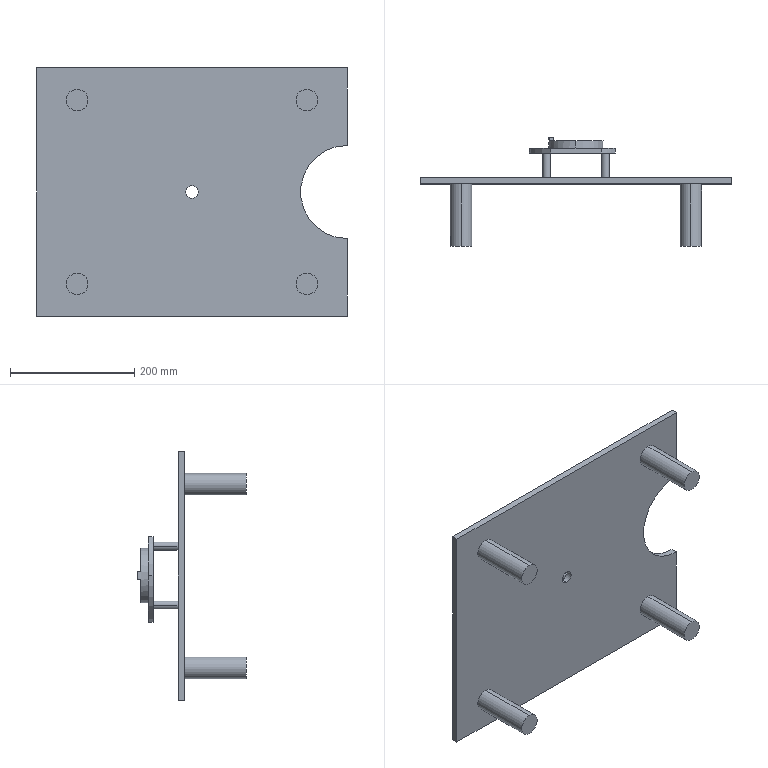Part | SolidWorks | features ICE 2, BaseBody 1 | 1 solid | 49 faces | box 500 x 175 x 400 mm | volume 2505450 mm3 | cylinder 29 | plane 20 | commonest cylinder face diameters 13 x8 35 x8 150 x4 20 x2 29 x2 30 x2
STEP:
#1=CARTESIAN_POINT('',(-15.,50.,0.6238));
#2=VERTEX_POINT('',#1);
#3=CARTESIAN_POINT('',(15.,50.,0.6238));
#4=VERTEX_POINT('',#3);
#5=CARTESIAN_POINT('',(0.,50.,0.6238));
#6=DIRECTION('',(0.,-1.,0.));
#7=DIRECTION('',(1.,0.,0.));
#8=AXIS2_PLACEMENT_3D('',#5,#6,#7);
#9=CIRCLE('',#8,15.);
#10=EDGE_CURVE('',#2,#4,#9,.T.);
#11=ORIENTED_EDGE('',*,*,#10,.T.);
#12=CARTESIAN_POINT('',(15.,58.,0.6238));
#13=VERTEX_POINT('',#12);
#14=CARTESIAN_POINT('',(15.,10.,0.6238));
#15=DIRECTION('',(0.,1.,0.));
#16=VECTOR('',#15,1000.);
#17=LINE('',#14,#16);
#18=EDGE_CURVE('',#4,#13,#17,.T.);
#19=ORIENTED_EDGE('',*,*,#18,.T.);
#20=CARTESIAN_POINT('',(-15.,58.,0.6238));
#21=VERTEX_POINT('',#20);
#22=CARTESIAN_POINT('',(0.,58.,0.6238));
#23=DIRECTION('',(0.,1.,0.));
#24=DIRECTION('',(-1.,0.,0.));
#25=AXIS2_PLACEMENT_3D('',#22,#23,#24);
#26=CIRCLE('',#25,15.);
#27=EDGE_CURVE('',#13,#21,#26,.T.);
#28=ORIENTED_EDGE('',*,*,#27,.T.);
#29=CARTESIAN_POINT('',(-15.,10.,0.6238));
#30=DIRECTION('',(0.,1.,0.));
#31=VECTOR('',#30,1000.);
#32=LINE('',#29,#31);
#33=EDGE_CURVE('',#2,#21,#32,.T.);
#34=ORIENTED_EDGE('',*,*,#33,.F.);
#35=EDGE_LOOP('',(#11,#19,#28,#34));
#36=FACE_OUTER_BOUND('',#35,.T.);
#37=CARTESIAN_POINT('',(0.,10.,0.6238));
#38=DIRECTION('',(0.,1.,0.));
#39=DIRECTION('',(-1.,0.,0.));
#40=AXIS2_PLACEMENT_3D('',#37,#38,#39);
#41=CYLINDRICAL_SURFACE('',#40,15.);
#42=ADVANCED_FACE('',(#36),#41,.F.);
#43=CARTESIAN_POINT('',(-40.876,10.,48.));
#44=VERTEX_POINT('',#43);
#45=CARTESIAN_POINT('',(-53.876,10.,48.));
#46=VERTEX_POINT('',#45);
#47=CARTESIAN_POINT('',(-47.376,10.,48.));
#48=DIRECTION('',(0.,-1.,0.));
#49=DIRECTION('',(1.,0.,0.));
#50=AXIS2_PLACEMENT_3D('',#47,#48,#49);
#51=CIRCLE('',#50,6.5);
#52=EDGE_CURVE('',#44,#46,#51,.T.);
#53=ORIENTED_EDGE('',*,*,#52,.F.);
#54=CARTESIAN_POINT('',(-40.876,50.,48.));
#55=VERTEX_POINT('',#54);
#56=CARTESIAN_POINT('',(-40.876,10.,48.));
#57=DIRECTION('',(0.,1.,0.));
#58=VECTOR('',#57,1000.);
#59=LINE('',#56,#58);
#60=EDGE_CURVE('',#44,#55,#59,.T.);
#61=ORIENTED_EDGE('',*,*,#60,.T.);
#62=CARTESIAN_POINT('',(-53.876,50.,48.));
#63=VERTEX_POINT('',#62);
#64=CARTESIAN_POINT('',(-47.376,50.,48.));
#65=DIRECTION('',(0.,-1.,0.));
#66=DIRECTION('',(1.,0.,0.));
#67=AXIS2_PLACEMENT_3D('',#64,#65,#66);
#68=CIRCLE('',#67,6.5);
#69=EDGE_CURVE('',#55,#63,#68,.T.);
#70=ORIENTED_EDGE('',*,*,#69,.T.);
#71=CARTESIAN_POINT('',(-53.876,10.,48.));
#72=DIRECTION('',(0.,1.,0.));
#73=VECTOR('',#72,1000.);
#74=LINE('',#71,#73);
#75=EDGE_CURVE('',#46,#63,#74,.T.);
#76=ORIENTED_EDGE('',*,*,#75,.F.);
#77=EDGE_LOOP('',(#53,#61,#70,#76));
#78=FACE_OUTER_BOUND('',#77,.T.);
#79=CARTESIAN_POINT('',(-47.376,10.,48.));
#80=DIRECTION('',(0.,1.,0.));
#81=DIRECTION('',(-1.,0.,0.));
#82=AXIS2_PLACEMENT_3D('',#79,#80,#81);
#83=CYLINDRICAL_SURFACE('',#82,6.5);
#84=ADVANCED_FACE('',(#78),#83,.T.);
#85=CARTESIAN_POINT('',(-75.,50.,0.6238));
#86=VERTEX_POINT('',#85);
#87=CARTESIAN_POINT('',(63.5,50.,-39.285));
#88=VERTEX_POINT('',#87);
#89=CARTESIAN_POINT('',(0.,50.,0.6238));
#90=DIRECTION('',(0.,-1.,0.));
#91=DIRECTION('',(1.,0.,0.));
#92=AXIS2_PLACEMENT_3D('',#89,#90,#91);
#93=CIRCLE('',#92,75.);
#94=EDGE_CURVE('',#86,#88,#93,.T.);
#95=ORIENTED_EDGE('',*,*,#94,.F.);
#96=CARTESIAN_POINT('',(-75.,58.,0.6238));
#97=VERTEX_POINT('',#96);
#98=CARTESIAN_POINT('',(-75.,50.,0.6238));
#99=DIRECTION('',(0.,1.,0.));
#100=VECTOR('',#99,1000.);
#101=LINE('',#98,#100);
#102=EDGE_CURVE('',#86,#97,#101,.T.);
#103=ORIENTED_EDGE('',*,*,#102,.T.);
#104=CARTESIAN_POINT('',(63.5,58.,-39.285));
#105=VERTEX_POINT('',#104);
#106=CARTESIAN_POINT('',(0.,58.,0.6238));
#107=DIRECTION('',(0.,-1.,0.));
#108=DIRECTION('',(1.,0.,0.));
#109=AXIS2_PLACEMENT_3D('',#106,#107,#108);
#110=CIRCLE('',#109,75.);
#111=EDGE_CURVE('',#97,#105,#110,.T.);
#112=ORIENTED_EDGE('',*,*,#111,.T.);
#113=CARTESIAN_POINT('',(63.5,50.,-39.285));
#114=DIRECTION('',(0.,-1.,0.));
#115=VECTOR('',#114,1000.);
#116=LINE('',#113,#115);
#117=EDGE_CURVE('',#105,#88,#116,.T.);
#118=ORIENTED_EDGE('',*,*,#117,.T.);
#119=EDGE_LOOP('',(#95,#103,#112,#118));
#120=FACE_OUTER_BOUND('',#119,.T.);
#121=CARTESIAN_POINT('',(0.,50.,0.6238));
#122=DIRECTION('',(0.,1.,0.));
#123=DIRECTION('',(-1.,0.,0.));
#124=AXIS2_PLACEMENT_3D('',#121,#122,#123);
#125=CYLINDRICAL_SURFACE('',#124,75.);
#126=ADVANCED_FACE('',(#120),#125,.T.);
#127=CARTESIAN_POINT('',(-40.876,10.,-46.752));
#128=VERTEX_POINT('',#127);
#129=CARTESIAN_POINT('',(-53.876,10.,-46.752));
#130=VERTEX_POINT('',#129);
#131=CARTESIAN_POINT('',(-47.376,10.,-46.752));
#132=DIRECTION('',(0.,-1.,0.));
#133=DIRECTION('',(0.,0.,1.));
#134=AXIS2_PLACEMENT_3D('',#131,#132,#133);
#135=CIRCLE('',#134,6.5);
#136=EDGE_CURVE('',#128,#130,#135,.T.);
#137=ORIENTED_EDGE('',*,*,#136,.F.);
#138=CARTESIAN_POINT('',(-40.876,50.,-46.752));
#139=VERTEX_POINT('',#138);
#140=CARTESIAN_POINT('',(-40.876,10.,-46.752));
#141=DIRECTION('',(0.,1.,0.));
#142=VECTOR('',#141,1000.);
#143=LINE('',#140,#142);
#144=EDGE_CURVE('',#128,#139,#143,.T.);
#145=ORIENTED_EDGE('',*,*,#144,.T.);
#146=CARTESIAN_POINT('',(-53.876,50.,-46.752));
#147=VERTEX_POINT('',#146);
#148=CARTESIAN_POINT('',(-47.376,50.,-46.752));
#149=DIRECTION('',(0.,-1.,0.));
#150=DIRECTION('',(0.,0.,1.));
#151=AXIS2_PLACEMENT_3D('',#148,#149,#150);
#152=CIRCLE('',#151,6.5);
#153=EDGE_CURVE('',#139,#147,#152,.T.);
#154=ORIENTED_EDGE('',*,*,#153,.T.);
#155=CARTESIAN_POINT('',(-53.876,10.,-46.752));
#156=DIRECTION('',(0.,1.,0.));
#157=VECTOR('',#156,1000.);
#158=LINE('',#155,#157);
#159=EDGE_CURVE('',#130,#147,#158,.T.);
#160=ORIENTED_EDGE('',*,*,#159,.F.);
#161=EDGE_LOOP('',(#137,#145,#154,#160));
#162=FACE_OUTER_BOUND('',#161,.T.);
#163=CARTESIAN_POINT('',(-47.376,10.,-46.752));
#164=DIRECTION('',(0.,1.,0.));
#165=DIRECTION('',(-1.,0.,0.));
#166=AXIS2_PLACEMENT_3D('',#163,#164,#165);
#167=CYLINDRICAL_SURFACE('',#166,6.5);
#168=ADVANCED_FACE('',(#162),#167,.T.);
#169=CARTESIAN_POINT('',(53.876,10.,-46.752));
#170=VERTEX_POINT('',#169);
#171=CARTESIAN_POINT('',(40.876,10.,-46.752));
#172=VERTEX_POINT('',#171);
#173=CARTESIAN_POINT('',(47.376,10.,-46.752));
#174=DIRECTION('',(0.,-1.,0.));
#175=DIRECTION('',(-1.,0.,0.));
#176=AXIS2_PLACEMENT_3D('',#173,#174,#175);
#177=CIRCLE('',#176,6.5);
#178=EDGE_CURVE('',#170,#172,#177,.T.);
#179=ORIENTED_EDGE('',*,*,#178,.F.);
#180=CARTESIAN_POINT('',(53.876,50.,-46.752));
#181=VERTEX_POINT('',#180);
#182=CARTESIAN_POINT('',(53.876,10.,-46.752));
#183=DIRECTION('',(0.,1.,0.));
#184=VECTOR('',#183,1000.);
#185=LINE('',#182,#184);
#186=EDGE_CURVE('',#170,#181,#185,.T.);
#187=ORIENTED_EDGE('',*,*,#186,.T.);
#188=CARTESIAN_POINT('',(40.876,50.,-46.752));
#189=VERTEX_POINT('',#188);
#190=CARTESIAN_POINT('',(47.376,50.,-46.752));
#191=DIRECTION('',(0.,-1.,0.));
#192=DIRECTION('',(-1.,0.,0.));
#193=AXIS2_PLACEMENT_3D('',#190,#191,#192);
#194=CIRCLE('',#193,6.5);
#195=EDGE_CURVE('',#181,#189,#194,.T.);
#196=ORIENTED_EDGE('',*,*,#195,.T.);
#197=CARTESIAN_POINT('',(40.876,10.,-46.752));
#198=DIRECTION('',(0.,1.,0.));
#199=VECTOR('',#198,1000.);
#200=LINE('',#197,#199);
#201=EDGE_CURVE('',#172,#189,#200,.T.);
#202=ORIENTED_EDGE('',*,*,#201,.F.);
#203=EDGE_LOOP('',(#179,#187,#196,#202));
#204=FACE_OUTER_BOUND('',#203,.T.);
#205=CARTESIAN_POINT('',(47.376,10.,-46.752));
#206=DIRECTION('',(0.,1.,0.));
#207=DIRECTION('',(-1.,0.,0.));
#208=AXIS2_PLACEMENT_3D('',#205,#206,#207);
#209=CYLINDRICAL_SURFACE('',#208,6.5);
#210=ADVANCED_FACE('',(#204),#209,.T.);
#211=CARTESIAN_POINT('',(53.876,10.,48.));
#212=VERTEX_POINT('',#211);
#213=CARTESIAN_POINT('',(40.876,10.,48.));
#214=VERTEX_POINT('',#213);
#215=CARTESIAN_POINT('',(47.376,10.,48.));
#216=DIRECTION('',(0.,-1.,0.));
#217=DIRECTION('',(0.,0.,-1.));
#218=AXIS2_PLACEMENT_3D('',#215,#216,#217);
#219=CIRCLE('',#218,6.5);
#220=EDGE_CURVE('',#212,#214,#219,.T.);
#221=ORIENTED_EDGE('',*,*,#220,.F.);
#222=CARTESIAN_POINT('',(53.876,50.,48.));
#223=VERTEX_POINT('',#222);
#224=CARTESIAN_POINT('',(53.876,10.,48.));
#225=DIRECTION('',(0.,1.,0.));
#226=VECTOR('',#225,1000.);
#227=LINE('',#224,#226);
#228=EDGE_CURVE('',#212,#223,#227,.T.);
#229=ORIENTED_EDGE('',*,*,#228,.T.);
#230=CARTESIAN_POINT('',(40.876,50.,48.));
#231=VERTEX_POINT('',#230);
#232=CARTESIAN_POINT('',(47.376,50.,48.));
#233=DIRECTION('',(0.,-1.,0.));
#234=DIRECTION('',(0.,0.,-1.));
#235=AXIS2_PLACEMENT_3D('',#232,#233,#234);
#236=CIRCLE('',#235,6.5);
#237=EDGE_CURVE('',#223,#231,#236,.T.);
#238=ORIENTED_EDGE('',*,*,#237,.T.);
#239=CARTESIAN_POINT('',(40.876,10.,48.));
#240=DIRECTION('',(0.,1.,0.));
#241=VECTOR('',#240,1000.);
#242=LINE('',#239,#241);
#243=EDGE_CURVE('',#214,#231,#242,.T.);
#244=ORIENTED_EDGE('',*,*,#243,.F.);
#245=EDGE_LOOP('',(#221,#229,#238,#244));
#246=FACE_OUTER_BOUND('',#245,.T.);
#247=CARTESIAN_POINT('',(47.376,10.,48.));
#248=DIRECTION('',(0.,1.,0.));
#249=DIRECTION('',(-1.,0.,0.));
#250=AXIS2_PLACEMENT_3D('',#247,#248,#249);
#251=CYLINDRICAL_SURFACE('',#250,6.5);
#252=ADVANCED_FACE('',(#246),#251,.T.);
#253=CARTESIAN_POINT('',(0.,0.,10.));
#254=VERTEX_POINT('',#253);
#255=CARTESIAN_POINT('',(0.,0.,-10.));
#256=VERTEX_POINT('',#255);
#257=CARTESIAN_POINT('',(0.,0.,0.));
#258=DIRECTION('',(0.,-1.,0.));
#259=DIRECTION('',(0.,0.,-1.));
#260=AXIS2_PLACEMENT_3D('',#257,#258,#259);
#261=CIRCLE('',#260,10.);
#262=EDGE_CURVE('',#254,#256,#261,.T.);
#263=ORIENTED_EDGE('',*,*,#262,.T.);
#264=CARTESIAN_POINT('',(0.,10.,-10.));
#265=VERTEX_POINT('',#264);
#266=CARTESIAN_POINT('',(0.,-100.,-10.));
#267=DIRECTION('',(0.,1.,0.));
#268=VECTOR('',#267,1000.);
#269=LINE('',#266,#268);
#270=EDGE_CURVE('',#256,#265,#269,.T.);
#271=ORIENTED_EDGE('',*,*,#270,.T.);
#272=CARTESIAN_POINT('',(0.,10.,10.));
#273=VERTEX_POINT('',#272);
#274=CARTESIAN_POINT('',(0.,10.,0.));
#275=DIRECTION('',(0.,1.,0.));
#276=DIRECTION('',(0.,0.,1.));
#277=AXIS2_PLACEMENT_3D('',#274,#275,#276);
#278=CIRCLE('',#277,10.);
#279=EDGE_CURVE('',#265,#273,#278,.T.);
#280=ORIENTED_EDGE('',*,*,#279,.T.);
#281=CARTESIAN_POINT('',(0.,-100.,10.));
#282=DIRECTION('',(0.,1.,0.));
#283=VECTOR('',#282,1000.);
#284=LINE('',#281,#283);
#285=EDGE_CURVE('',#254,#273,#284,.T.);
#286=ORIENTED_EDGE('',*,*,#285,.F.);
#287=EDGE_LOOP('',(#263,#271,#280,#286));
#288=FACE_OUTER_BOUND('',#287,.T.);
#289=CARTESIAN_POINT('',(0.,-100.,0.));
#290=DIRECTION('',(0.,1.,0.));
#291=DIRECTION('',(0.,0.,1.));
#292=AXIS2_PLACEMENT_3D('',#289,#290,#291);
#293=CYLINDRICAL_SURFACE('',#292,10.);
#294=ADVANCED_FACE('',(#288),#293,.F.);
#295=CARTESIAN_POINT('',(-185.,-100.,165.5));
#296=VERTEX_POINT('',#295);
#297=CARTESIAN_POINT('',(-185.,-100.,130.5));
#298=VERTEX_POINT('',#297);
#299=CARTESIAN_POINT('',(-185.,-100.,148.));
#300=DIRECTION('',(0.,1.,0.));
#301=DIRECTION('',(0.,0.,1.));
#302=AXIS2_PLACEMENT_3D('',#299,#300,#301);
#303=CIRCLE('',#302,17.5);
#304=EDGE_CURVE('',#296,#298,#303,.T.);
#305=ORIENTED_EDGE('',*,*,#304,.T.);
#306=CARTESIAN_POINT('',(-185.,0.,130.5));
#307=VERTEX_POINT('',#306);
#308=CARTESIAN_POINT('',(-185.,-100.,130.5));
#309=DIRECTION('',(0.,1.,0.));
#310=VECTOR('',#309,1000.);
#311=LINE('',#308,#310);
#312=EDGE_CURVE('',#298,#307,#311,.T.);
#313=ORIENTED_EDGE('',*,*,#312,.T.);
#314=CARTESIAN_POINT('',(-185.,0.,165.5));
#315=VERTEX_POINT('',#314);
#316=CARTESIAN_POINT('',(-185.,0.,148.));
#317=DIRECTION('',(0.,-1.,0.));
#318=DIRECTION('',(0.,0.,-1.));
#319=AXIS2_PLACEMENT_3D('',#316,#317,#318);
#320=CIRCLE('',#319,17.5);
#321=EDGE_CURVE('',#307,#315,#320,.T.);
#322=ORIENTED_EDGE('',*,*,#321,.T.);
#323=CARTESIAN_POINT('',(-185.,-100.,165.5));
#324=DIRECTION('',(0.,1.,0.));
#325=VECTOR('',#324,1000.);
#326=LINE('',#323,#325);
#327=EDGE_CURVE('',#296,#315,#326,.T.);
#328=ORIENTED_EDGE('',*,*,#327,.F.);
#329=EDGE_LOOP('',(#305,#313,#322,#328));
#330=FACE_OUTER_BOUND('',#329,.T.);
#331=CARTESIAN_POINT('',(-185.,-100.,148.));
#332=DIRECTION('',(0.,1.,0.));
#333=DIRECTION('',(0.,0.,1.));
#334=AXIS2_PLACEMENT_3D('',#331,#332,#333);
#335=CYLINDRICAL_SURFACE('',#334,17.5);
#336=ADVANCED_FACE('',(#330),#335,.T.);
#337=CARTESIAN_POINT('',(185.,-100.,130.5));
#338=VERTEX_POINT('',#337);
#339=CARTESIAN_POINT('',(185.,-100.,165.5));
#340=VERTEX_POINT('',#339);
#341=CARTESIAN_POINT('',(185.,-100.,148.));
#342=DIRECTION('',(0.,-1.,0.));
#343=DIRECTION('',(0.,0.,1.));
#344=AXIS2_PLACEMENT_3D('',#341,#342,#343);
#345=CIRCLE('',#344,17.5);
#346=EDGE_CURVE('',#338,#340,#345,.T.);
#347=ORIENTED_EDGE('',*,*,#346,.F.);
#348=CARTESIAN_POINT('',(185.,0.,130.5));
#349=VERTEX_POINT('',#348);
#350=CARTESIAN_POINT('',(185.,-100.,130.5));
#351=DIRECTION('',(0.,1.,0.));
#352=VECTOR('',#351,1000.);
#353=LINE('',#350,#352);
#354=EDGE_CURVE('',#338,#349,#353,.T.);
#355=ORIENTED_EDGE('',*,*,#354,.T.);
#356=CARTESIAN_POINT('',(185.,0.,165.5));
#357=VERTEX_POINT('',#356);
#358=CARTESIAN_POINT('',(185.,0.,148.));
#359=DIRECTION('',(0.,-1.,0.));
#360=DIRECTION('',(0.,0.,1.));
#361=AXIS2_PLACEMENT_3D('',#358,#359,#360);
#362=CIRCLE('',#361,17.5);
#363=EDGE_CURVE('',#349,#357,#362,.T.);
#364=ORIENTED_EDGE('',*,*,#363,.T.);
#365=CARTESIAN_POINT('',(185.,-100.,165.5));
#366=DIRECTION('',(0.,1.,0.));
#367=VECTOR('',#366,1000.);
#368=LINE('',#365,#367);
#369=EDGE_CURVE('',#340,#357,#368,.T.);
#370=ORIENTED_EDGE('',*,*,#369,.F.);
#371=EDGE_LOOP('',(#347,#355,#364,#370));
#372=FACE_OUTER_BOUND('',#371,.T.);
#373=CARTESIAN_POINT('',(185.,-100.,148.));
#374=DIRECTION('',(0.,1.,0.));
#375=DIRECTION('',(0.,0.,1.));
#376=AXIS2_PLACEMENT_3D('',#373,#374,#375);
#377=CYLINDRICAL_SURFACE('',#376,17.5);
#378=ADVANCED_FACE('',(#372),#377,.T.);
#379=CARTESIAN_POINT('',(185.,-100.,-130.5));
#380=VERTEX_POINT('',#379);
#381=CARTESIAN_POINT('',(185.,-100.,-165.5));
#382=VERTEX_POINT('',#381);
#383=CARTESIAN_POINT('',(185.,-100.,-148.));
#384=DIRECTION('',(0.,1.,0.));
#385=DIRECTION('',(0.,0.,-1.));
#386=AXIS2_PLACEMENT_3D('',#383,#384,#385);
#387=CIRCLE('',#386,17.5);
#388=EDGE_CURVE('',#380,#382,#387,.T.);
#389=ORIENTED_EDGE('',*,*,#388,.T.);
#390=CARTESIAN_POINT('',(185.,0.,-165.5));
#391=VERTEX_POINT('',#390);
#392=CARTESIAN_POINT('',(185.,-100.,-165.5));
#393=DIRECTION('',(0.,1.,0.));
#394=VECTOR('',#393,1000.);
#395=LINE('',#392,#394);
#396=EDGE_CURVE('',#382,#391,#395,.T.);
#397=ORIENTED_EDGE('',*,*,#396,.T.);
#398=CARTESIAN_POINT('',(185.,0.,-130.5));
#399=VERTEX_POINT('',#398);
#400=CARTESIAN_POINT('',(185.,0.,-148.));
#401=DIRECTION('',(0.,-1.,0.));
#402=DIRECTION('',(0.,0.,-1.));
#403=AXIS2_PLACEMENT_3D('',#400,#401,#402);
#404=CIRCLE('',#403,17.5);
#405=EDGE_CURVE('',#391,#399,#404,.T.);
#406=ORIENTED_EDGE('',*,*,#405,.T.);
#407=CARTESIAN_POINT('',(185.,-100.,-130.5));
#408=DIRECTION('',(0.,1.,0.));
#409=VECTOR('',#408,1000.);
#410=LINE('',#407,#409);
#411=EDGE_CURVE('',#380,#399,#410,.T.);
#412=ORIENTED_EDGE('',*,*,#411,.F.);
#413=EDGE_LOOP('',(#389,#397,#406,#412));
#414=FACE_OUTER_BOUND('',#413,.T.);
#415=CARTESIAN_POINT('',(185.,-100.,-148.));
#416=DIRECTION('',(0.,1.,0.));
#417=DIRECTION('',(0.,0.,1.));
#418=AXIS2_PLACEMENT_3D('',#415,#416,#417);
#419=CYLINDRICAL_SURFACE('',#418,17.5);
#420=ADVANCED_FACE('',(#414),#419,.T.);
#421=CARTESIAN_POINT('',(-185.,-100.,-165.5));
#422=VERTEX_POINT('',#421);
#423=CARTESIAN_POINT('',(-185.,-100.,-130.5));
#424=VERTEX_POINT('',#423);
#425=CARTESIAN_POINT('',(-185.,-100.,-148.));
#426=DIRECTION('',(0.,-1.,0.));
#427=DIRECTION('',(0.,0.,-1.));
#428=AXIS2_PLACEMENT_3D('',#425,#426,#427);
#429=CIRCLE('',#428,17.5);
#430=EDGE_CURVE('',#422,#424,#429,.T.);
#431=ORIENTED_EDGE('',*,*,#430,.F.);
#432=CARTESIAN_POINT('',(-185.,0.,-165.5));
#433=VERTEX_POINT('',#432);
#434=CARTESIAN_POINT('',(-185.,-100.,-165.5));
#435=DIRECTION('',(0.,1.,0.));
#436=VECTOR('',#435,1000.);
#437=LINE('',#434,#436);
#438=EDGE_CURVE('',#422,#433,#437,.T.);
#439=ORIENTED_EDGE('',*,*,#438,.T.);
#440=CARTESIAN_POINT('',(-185.,0.,-130.5));
#441=VERTEX_POINT('',#440);
#442=CARTESIAN_POINT('',(-185.,0.,-148.));
#443=DIRECTION('',(0.,-1.,0.));
#444=DIRECTION('',(0.,0.,-1.));
#445=AXIS2_PLACEMENT_3D('',#442,#443,#444);
#446=CIRCLE('',#445,17.5);
#447=EDGE_CURVE('',#433,#441,#446,.T.);
#448=ORIENTED_EDGE('',*,*,#447,.T.);
#449=CARTESIAN_POINT('',(-185.,-100.,-130.5));
#450=DIRECTION('',(0.,1.,0.));
#451=VECTOR('',#450,1000.);
#452=LINE('',#449,#451);
#453=EDGE_CURVE('',#424,#441,#452,.T.);
#454=ORIENTED_EDGE('',*,*,#453,.F.);
#455=EDGE_LOOP('',(#431,#439,#448,#454));
#456=FACE_OUTER_BOUND('',#455,.T.);
#457=CARTESIAN_POINT('',(-185.,-100.,-148.));
#458=DIRECTION('',(0.,1.,0.));
#459=DIRECTION('',(0.,0.,1.));
#460=AXIS2_PLACEMENT_3D('',#457,#458,#459);
#461=CYLINDRICAL_SURFACE('',#460,17.5);
#462=ADVANCED_FACE('',(#456),#461,.T.);
#463=CARTESIAN_POINT('',(0.,70.,15.124));
#464=VERTEX_POINT('',#463);
#465=CARTESIAN_POINT('',(0.,70.,-13.876));
#466=VERTEX_POINT('',#465);
#467=CARTESIAN_POINT('',(0.,70.,0.6238));
#468=DIRECTION('',(0.,-1.,0.));
#469=DIRECTION('',(0.,0.,-1.));
#470=AXIS2_PLACEMENT_3D('',#467,#468,#469);
#471=CIRCLE('',#470,14.5);
#472=EDGE_CURVE('',#464,#466,#471,.T.);
#473=ORIENTED_EDGE('',*,*,#472,.F.);
#474=CARTESIAN_POINT('',(0.,58.,15.124));
#475=VERTEX_POINT('',#474);
#476=CARTESIAN_POINT('',(0.,58.,15.124));
#477=DIRECTION('',(0.,-1.,0.));
#478=VECTOR('',#477,1000.);
#479=LINE('',#476,#478);
#480=EDGE_CURVE('',#464,#475,#479,.T.);
#481=ORIENTED_EDGE('',*,*,#480,.T.);
#482=CARTESIAN_POINT('',(0.,58.,-13.876));
#483=VERTEX_POINT('',#482);
#484=CARTESIAN_POINT('',(0.,58.,0.6238));
#485=DIRECTION('',(0.,-1.,0.));
#486=DIRECTION('',(0.,0.,-1.));
#487=AXIS2_PLACEMENT_3D('',#484,#485,#486);
#488=CIRCLE('',#487,14.5);
#489=EDGE_CURVE('',#475,#483,#488,.T.);
#490=ORIENTED_EDGE('',*,*,#489,.T.);
#491=CARTESIAN_POINT('',(0.,58.,-13.876));
#492=DIRECTION('',(0.,-1.,0.));
#493=VECTOR('',#492,1000.);
#494=LINE('',#491,#493);
#495=EDGE_CURVE('',#466,#483,#494,.T.);
#496=ORIENTED_EDGE('',*,*,#495,.F.);
#497=EDGE_LOOP('',(#473,#481,#490,#496));
#498=FACE_OUTER_BOUND('',#497,.T.);
#499=CARTESIAN_POINT('',(0.,58.,0.6238));
#500=DIRECTION('',(0.,-1.,0.));
#501=DIRECTION('',(0.,0.,-1.));
#502=AXIS2_PLACEMENT_3D('',#499,#500,#501);
#503=CYLINDRICAL_SURFACE('',#502,14.5);
#504=ADVANCED_FACE('',(#498),#503,.F.);
#505=CARTESIAN_POINT('',(0.,70.,-43.376));
#506=VERTEX_POINT('',#505);
#507=CARTESIAN_POINT('',(0.,70.,44.624));
#508=VERTEX_POINT('',#507);
#509=CARTESIAN_POINT('',(0.,70.,0.6238));
#510=DIRECTION('',(0.,-1.,0.));
#511=DIRECTION('',(0.,0.,-1.));
#512=AXIS2_PLACEMENT_3D('',#509,#510,#511);
#513=CIRCLE('',#512,44.);
#514=EDGE_CURVE('',#506,#508,#513,.T.);
#515=ORIENTED_EDGE('',*,*,#514,.T.);
#516=CARTESIAN_POINT('',(0.,58.,44.624));
#517=VERTEX_POINT('',#516);
#518=CARTESIAN_POINT('',(0.,58.,44.624));
#519=DIRECTION('',(0.,-1.,0.));
#520=VECTOR('',#519,1000.);
#521=LINE('',#518,#520);
#522=EDGE_CURVE('',#508,#517,#521,.T.);
#523=ORIENTED_EDGE('',*,*,#522,.T.);
#524=CARTESIAN_POINT('',(0.,58.,-43.376));
#525=VERTEX_POINT('',#524);
#526=CARTESIAN_POINT('',(0.,58.,0.6238));
#527=DIRECTION('',(0.,-1.,0.));
#528=DIRECTION('',(0.,0.,-1.));
#529=AXIS2_PLACEMENT_3D('',#526,#527,#528);
#530=CIRCLE('',#529,44.);
#531=EDGE_CURVE('',#525,#517,#530,.T.);
#532=ORIENTED_EDGE('',*,*,#531,.F.);
#533=CARTESIAN_POINT('',(0.,58.,-43.376));
#534=DIRECTION('',(0.,-1.,0.));
#535=VECTOR('',#534,1000.);
#536=LINE('',#533,#535);
#537=EDGE_CURVE('',#506,#525,#536,.T.);
#538=ORIENTED_EDGE('',*,*,#537,.F.);
#539=EDGE_LOOP('',(#515,#523,#532,#538));
#540=FACE_OUTER_BOUND('',#539,.T.);
#541=CARTESIAN_POINT('',(0.,58.,0.6238));
#542=DIRECTION('',(0.,-1.,0.));
#543=DIRECTION('',(0.,0.,-1.));
#544=AXIS2_PLACEMENT_3D('',#541,#542,#543);
#545=CYLINDRICAL_SURFACE('',#544,44.);
#546=ADVANCED_FACE('',(#540),#545,.T.);
#547=CARTESIAN_POINT('',(250.,0.,200.));
#548=VERTEX_POINT('',#547);
#549=CARTESIAN_POINT('',(250.,0.,75.));
#550=VERTEX_POINT('',#549);
#551=CARTESIAN_POINT('',(250.,0.,-200.));
#552=DIRECTION('',(0.,0.,-1.));
#553=VECTOR('',#552,1000.);
#554=LINE('',#551,#553);
#555=EDGE_CURVE('',#548,#550,#554,.T.);
#556=ORIENTED_EDGE('',*,*,#555,.T.);
#557=CARTESIAN_POINT('',(250.,10.,75.));
#558=VERTEX_POINT('',#557);
#559=CARTESIAN_POINT('',(250.,-100.,75.));
#560=DIRECTION('',(0.,1.,0.));
#561=VECTOR('',#560,1000.);
#562=LINE('',#559,#561);
#563=EDGE_CURVE('',#550,#558,#562,.T.);
#564=ORIENTED_EDGE('',*,*,#563,.T.);
#565=CARTESIAN_POINT('',(250.,10.,200.));
#566=VERTEX_POINT('',#565);
#567=CARTESIAN_POINT('',(250.,10.,200.));
#568=DIRECTION('',(0.,0.,-1.));
#569=VECTOR('',#568,1000.);
#570=LINE('',#567,#569);
#571=EDGE_CURVE('',#566,#558,#570,.T.);
#572=ORIENTED_EDGE('',*,*,#571,.F.);
#573=CARTESIAN_POINT('',(250.,4.,200.));
#574=DIRECTION('',(0.,-1.,0.));
#575=VECTOR('',#574,1000.);
#576=LINE('',#573,#575);
#577=EDGE_CURVE('',#566,#548,#576,.T.);
#578=ORIENTED_EDGE('',*,*,#577,.T.);
#579=EDGE_LOOP('',(#556,#564,#572,#578));
#580=FACE_OUTER_BOUND('',#579,.T.);
#581=CARTESIAN_POINT('',(250.,4.,-200.));
#582=DIRECTION('',(-1.,0.,0.));
#583=DIRECTION('',(0.,0.,1.));
#584=AXIS2_PLACEMENT_3D('',#581,#582,#583);
#585=PLANE('',#584);
#586=ADVANCED_FACE('',(#580),#585,.F.);
#587=CARTESIAN_POINT('',(63.5,50.,40.533));
#588=VERTEX_POINT('',#587);
#589=CARTESIAN_POINT('',(40.885,50.,63.5));
#590=VERTEX_POINT('',#589);
#591=CARTESIAN_POINT('',(0.,50.,0.6238));
#592=DIRECTION('',(0.,-1.,0.));
#593=DIRECTION('',(1.,0.,0.));
#594=AXIS2_PLACEMENT_3D('',#591,#592,#593);
#595=CIRCLE('',#594,75.);
#596=EDGE_CURVE('',#588,#590,#595,.T.);
#597=ORIENTED_EDGE('',*,*,#596,.F.);
#598=CARTESIAN_POINT('',(63.5,58.,40.533));
#599=VERTEX_POINT('',#598);
#600=CARTESIAN_POINT('',(63.5,50.,40.533));
#601=DIRECTION('',(0.,1.,0.));
#602=VECTOR('',#601,1000.);
#603=LINE('',#600,#602);
#604=EDGE_CURVE('',#588,#599,#603,.T.);
#605=ORIENTED_EDGE('',*,*,#604,.T.);
#606=CARTESIAN_POINT('',(40.885,58.,63.5));
#607=VERTEX_POINT('',#606);
#608=CARTESIAN_POINT('',(0.,58.,0.6238));
#609=DIRECTION('',(0.,-1.,0.));
#610=DIRECTION('',(1.,0.,0.));
#611=AXIS2_PLACEMENT_3D('',#608,#609,#610);
#612=CIRCLE('',#611,75.);
#613=EDGE_CURVE('',#599,#607,#612,.T.);
#614=ORIENTED_EDGE('',*,*,#613,.T.);
#615=CARTESIAN_POINT('',(40.885,50.,63.5));
#616=DIRECTION('',(0.,-1.,0.));
#617=VECTOR('',#616,1000.);
#618=LINE('',#615,#617);
#619=EDGE_CURVE('',#607,#590,#618,.T.);
#620=ORIENTED_EDGE('',*,*,#619,.T.);
#621=EDGE_LOOP('',(#597,#605,#614,#620));
#622=FACE_OUTER_BOUND('',#621,.T.);
#623=CARTESIAN_POINT('',(0.,50.,0.6238));
#624=DIRECTION('',(0.,1.,0.));
#625=DIRECTION('',(-1.,0.,0.));
#626=AXIS2_PLACEMENT_3D('',#623,#624,#625);
#627=CYLINDRICAL_SURFACE('',#626,75.);
#628=ADVANCED_FACE('',(#622),#627,.T.);
#629=CARTESIAN_POINT('',(0.,58.,0.6238));
#630=DIRECTION('',(0.,-1.,0.));
#631=DIRECTION('',(0.,0.,-1.));
#632=AXIS2_PLACEMENT_3D('',#629,#630,#631);
#633=CIRCLE('',#632,14.5);
#634=EDGE_CURVE('',#483,#475,#633,.T.);
#635=ORIENTED_EDGE('',*,*,#634,.F.);
#636=ORIENTED_EDGE('',*,*,#489,.F.);
#637=EDGE_LOOP('',(#635,#636));
#638=FACE_BOUND('',#637,.T.);
#639=CARTESIAN_POINT('',(0.,58.,0.6238));
#640=DIRECTION('',(0.,1.,0.));
#641=DIRECTION('',(-1.,0.,0.));
#642=AXIS2_PLACEMENT_3D('',#639,#640,#641);
#643=CIRCLE('',#642,15.);
#644=EDGE_CURVE('',#21,#13,#643,.T.);
#645=ORIENTED_EDGE('',*,*,#644,.F.);
#646=ORIENTED_EDGE('',*,*,#27,.F.);
#647=EDGE_LOOP('',(#645,#646));
#648=FACE_OUTER_BOUND('',#647,.T.);
#649=CARTESIAN_POINT('',(14.5,58.,0.6238));
#650=DIRECTION('',(0.,-1.,0.));
#651=DIRECTION('',(0.,0.,-1.));
#652=AXIS2_PLACEMENT_3D('',#649,#650,#651);
#653=PLANE('',#652);
#654=ADVANCED_FACE('',(#638,#648),#653,.T.);
#655=ORIENTED_EDGE('',*,*,#522,.F.);
#656=CARTESIAN_POINT('',(-43.458,70.,7.507));
#657=VERTEX_POINT('',#656);
#658=CARTESIAN_POINT('',(0.,70.,0.6238));
#659=DIRECTION('',(0.,-1.,0.));
#660=DIRECTION('',(0.,0.,-1.));
#661=AXIS2_PLACEMENT_3D('',#658,#659,#660);
#662=CIRCLE('',#661,44.);
#663=EDGE_CURVE('',#508,#657,#662,.T.);
#664=ORIENTED_EDGE('',*,*,#663,.T.);
#665=CARTESIAN_POINT('',(-43.458,75.,7.507));
#666=VERTEX_POINT('',#665);
#667=CARTESIAN_POINT('',(-43.458,75.,7.507));
#668=DIRECTION('',(0.,-1.,0.));
#669=VECTOR('',#668,1000.);
#670=LINE('',#667,#669);
#671=EDGE_CURVE('',#666,#657,#670,.T.);
#672=ORIENTED_EDGE('',*,*,#671,.F.);
#673=CARTESIAN_POINT('',(-43.458,75.,-6.259));
#674=VERTEX_POINT('',#673);
#675=CARTESIAN_POINT('',(0.,75.,0.6238));
#676=DIRECTION('',(0.,1.,0.));
#677=DIRECTION('',(0.,0.,1.));
#678=AXIS2_PLACEMENT_3D('',#675,#676,#677);
#679=CIRCLE('',#678,44.);
#680=EDGE_CURVE('',#674,#666,#679,.T.);
#681=ORIENTED_EDGE('',*,*,#680,.F.);
#682=CARTESIAN_POINT('',(-43.458,70.,-6.259));
#683=VERTEX_POINT('',#682);
#684=CARTESIAN_POINT('',(-43.458,75.,-6.259));
#685=DIRECTION('',(0.,-1.,0.));
#686=VECTOR('',#685,1000.);
#687=LINE('',#684,#686);
#688=EDGE_CURVE('',#674,#683,#687,.T.);
#689=ORIENTED_EDGE('',*,*,#688,.T.);
#690=CARTESIAN_POINT('',(0.,70.,0.6238));
#691=DIRECTION('',(0.,-1.,0.));
#692=DIRECTION('',(0.,0.,-1.));
#693=AXIS2_PLACEMENT_3D('',#690,#691,#692);
#694=CIRCLE('',#693,44.);
#695=EDGE_CURVE('',#683,#506,#694,.T.);
#696=ORIENTED_EDGE('',*,*,#695,.T.);
#697=ORIENTED_EDGE('',*,*,#537,.T.);
#698=CARTESIAN_POINT('',(0.,58.,0.6238));
#699=DIRECTION('',(0.,-1.,0.));
#700=DIRECTION('',(0.,0.,-1.));
#701=AXIS2_PLACEMENT_3D('',#698,#699,#700);
#702=CIRCLE('',#701,44.);
#703=EDGE_CURVE('',#517,#525,#702,.T.);
#704=ORIENTED_EDGE('',*,*,#703,.F.);
#705=EDGE_LOOP('',(#655,#664,#672,#681,#689,#696,#697,#704));
#706=FACE_OUTER_BOUND('',#705,.T.);
#707=CARTESIAN_POINT('',(0.,58.,0.6238));
#708=DIRECTION('',(0.,-1.,0.));
#709=DIRECTION('',(0.,0.,-1.));
#710=AXIS2_PLACEMENT_3D('',#707,#708,#709);
#711=CYLINDRICAL_SURFACE('',#710,44.);
#712=ADVANCED_FACE('',(#706),#711,.T.);
#713=ORIENTED_EDGE('',*,*,#480,.F.);
#714=CARTESIAN_POINT('',(0.,70.,0.6238));
#715=DIRECTION('',(0.,-1.,0.));
#716=DIRECTION('',(0.,0.,-1.));
#717=AXIS2_PLACEMENT_3D('',#714,#715,#716);
#718=CIRCLE('',#717,14.5);
#719=EDGE_CURVE('',#466,#464,#718,.T.);
#720=ORIENTED_EDGE('',*,*,#719,.F.);
#721=ORIENTED_EDGE('',*,*,#495,.T.);
#722=ORIENTED_EDGE('',*,*,#634,.T.);
#723=EDGE_LOOP('',(#713,#720,#721,#722));
#724=FACE_OUTER_BOUND('',#723,.T.);
#725=CARTESIAN_POINT('',(0.,58.,0.6238));
#726=DIRECTION('',(0.,-1.,0.));
#727=DIRECTION('',(0.,0.,-1.));
#728=AXIS2_PLACEMENT_3D('',#725,#726,#727);
#729=CYLINDRICAL_SURFACE('',#728,14.5);
#730=ADVANCED_FACE('',(#724),#729,.F.);
#731=CARTESIAN_POINT('',(-36.544,70.,-5.164));
#732=VERTEX_POINT('',#731);
#733=CARTESIAN_POINT('',(0.,70.,0.6238));
#734=DIRECTION('',(-0.9877,0.,-0.1564));
#735=VECTOR('',#734,1000.);
#736=LINE('',#733,#735);
#737=EDGE_CURVE('',#732,#683,#736,.T.);
#738=ORIENTED_EDGE('',*,*,#737,.F.);
#739=CARTESIAN_POINT('',(-36.544,70.,6.412));
#740=VERTEX_POINT('',#739);
#741=CARTESIAN_POINT('',(0.,70.,0.6238));
#742=DIRECTION('',(0.,1.,0.));
#743=DIRECTION('',(0.,0.,1.));
#744=AXIS2_PLACEMENT_3D('',#741,#742,#743);
#745=CIRCLE('',#744,37.);
#746=EDGE_CURVE('',#732,#740,#745,.T.);
#747=ORIENTED_EDGE('',*,*,#746,.T.);
#748=CARTESIAN_POINT('',(0.,70.,0.6238));
#749=DIRECTION('',(-0.9877,0.,0.1564));
#750=VECTOR('',#749,1000.);
#751=LINE('',#748,#750);
#752=EDGE_CURVE('',#740,#657,#751,.T.);
#753=ORIENTED_EDGE('',*,*,#752,.T.);
#754=ORIENTED_EDGE('',*,*,#663,.F.);
#755=ORIENTED_EDGE('',*,*,#514,.F.);
#756=ORIENTED_EDGE('',*,*,#695,.F.);
#757=EDGE_LOOP('',(#738,#747,#753,#754,#755,#756));
#758=FACE_OUTER_BOUND('',#757,.T.);
#759=ORIENTED_EDGE('',*,*,#719,.T.);
#760=ORIENTED_EDGE('',*,*,#472,.T.);
#761=EDGE_LOOP('',(#759,#760));
#762=FACE_BOUND('',#761,.T.);
#763=CARTESIAN_POINT('',(14.5,70.,0.6238));
#764=DIRECTION('',(0.,1.,0.));
#765=DIRECTION('',(0.,0.,1.));
#766=AXIS2_PLACEMENT_3D('',#763,#764,#765);
#767=PLANE('',#766);
#768=ADVANCED_FACE('',(#758,#762),#767,.T.);
#769=ORIENTED_EDGE('',*,*,#752,.F.);
#770=CARTESIAN_POINT('',(-36.544,75.,6.412));
#771=VERTEX_POINT('',#770);
#772=CARTESIAN_POINT('',(-36.544,75.,6.412));
#773=DIRECTION('',(0.,-1.,0.));
#774=VECTOR('',#773,1000.);
#775=LINE('',#772,#774);
#776=EDGE_CURVE('',#771,#740,#775,.T.);
#777=ORIENTED_EDGE('',*,*,#776,.F.);
#778=CARTESIAN_POINT('',(0.,75.,0.6238));
#779=DIRECTION('',(-0.9877,0.,0.1564));
#780=VECTOR('',#779,1000.);
#781=LINE('',#778,#780);
#782=EDGE_CURVE('',#771,#666,#781,.T.);
#783=ORIENTED_EDGE('',*,*,#782,.T.);
#784=ORIENTED_EDGE('',*,*,#671,.T.);
#785=EDGE_LOOP('',(#769,#777,#783,#784));
#786=FACE_OUTER_BOUND('',#785,.T.);
#787=CARTESIAN_POINT('',(0.,75.,0.6238));
#788=DIRECTION('',(0.1564,0.,0.9877));
#789=DIRECTION('',(0.9877,0.,-0.1564));
#790=AXIS2_PLACEMENT_3D('',#787,#788,#789);
#791=PLANE('',#790);
#792=ADVANCED_FACE('',(#786),#791,.T.);
#793=ORIENTED_EDGE('',*,*,#746,.F.);
#794=CARTESIAN_POINT('',(-36.544,75.,-5.164));
#795=VERTEX_POINT('',#794);
#796=CARTESIAN_POINT('',(-36.544,75.,-5.164));
#797=DIRECTION('',(0.,-1.,0.));
#798=VECTOR('',#797,1000.);
#799=LINE('',#796,#798);
#800=EDGE_CURVE('',#795,#732,#799,.T.);
#801=ORIENTED_EDGE('',*,*,#800,.F.);
#802=CARTESIAN_POINT('',(0.,75.,0.6238));
#803=DIRECTION('',(0.,1.,0.));
#804=DIRECTION('',(0.,0.,1.));
#805=AXIS2_PLACEMENT_3D('',#802,#803,#804);
#806=CIRCLE('',#805,37.);
#807=EDGE_CURVE('',#795,#771,#806,.T.);
#808=ORIENTED_EDGE('',*,*,#807,.T.);
#809=ORIENTED_EDGE('',*,*,#776,.T.);
#810=EDGE_LOOP('',(#793,#801,#808,#809));
#811=FACE_OUTER_BOUND('',#810,.T.);
#812=CARTESIAN_POINT('',(0.,75.,0.6238));
#813=DIRECTION('',(0.,-1.,0.));
#814=DIRECTION('',(0.,0.,-1.));
#815=AXIS2_PLACEMENT_3D('',#812,#813,#814);
#816=CYLINDRICAL_SURFACE('',#815,37.);
#817=ADVANCED_FACE('',(#811),#816,.F.);
#818=ORIENTED_EDGE('',*,*,#737,.T.);
#819=ORIENTED_EDGE('',*,*,#688,.F.);
#820=CARTESIAN_POINT('',(0.,75.,0.6238));
#821=DIRECTION('',(-0.9877,0.,-0.1564));
#822=VECTOR('',#821,1000.);
#823=LINE('',#820,#822);
#824=EDGE_CURVE('',#795,#674,#823,.T.);
#825=ORIENTED_EDGE('',*,*,#824,.F.);
#826=ORIENTED_EDGE('',*,*,#800,.T.);
#827=EDGE_LOOP('',(#818,#819,#825,#826));
#828=FACE_OUTER_BOUND('',#827,.T.);
#829=CARTESIAN_POINT('',(0.,75.,0.6238));
#830=DIRECTION('',(-0.1564,0.,0.9877));
#831=DIRECTION('',(0.9877,0.,0.1564));
#832=AXIS2_PLACEMENT_3D('',#829,#830,#831);
#833=PLANE('',#832);
#834=ADVANCED_FACE('',(#828),#833,.F.);
#835=ORIENTED_EDGE('',*,*,#680,.T.);
#836=ORIENTED_EDGE('',*,*,#782,.F.);
#837=ORIENTED_EDGE('',*,*,#807,.F.);
#838=ORIENTED_EDGE('',*,*,#824,.T.);
#839=EDGE_LOOP('',(#835,#836,#837,#838));
#840=FACE_OUTER_BOUND('',#839,.T.);
#841=CARTESIAN_POINT('',(0.,75.,0.6238));
#842=DIRECTION('',(0.,1.,0.));
#843=DIRECTION('',(0.,0.,1.));
#844=AXIS2_PLACEMENT_3D('',#841,#842,#843);
#845=PLANE('',#844);
#846=ADVANCED_FACE('',(#840),#845,.T.);
#847=ORIENTED_EDGE('',*,*,#613,.F.);
#848=CARTESIAN_POINT('',(63.5,58.,-50.8));
#849=DIRECTION('',(0.,0.,1.));
#850=VECTOR('',#849,1000.);
#851=LINE('',#848,#850);
#852=EDGE_CURVE('',#105,#599,#851,.T.);
#853=ORIENTED_EDGE('',*,*,#852,.F.);
#854=ORIENTED_EDGE('',*,*,#111,.F.);
#855=CARTESIAN_POINT('',(-40.885,58.,63.5));
#856=VERTEX_POINT('',#855);
#857=CARTESIAN_POINT('',(0.,58.,0.6238));
#858=DIRECTION('',(0.,-1.,0.));
#859=DIRECTION('',(1.,0.,0.));
#860=AXIS2_PLACEMENT_3D('',#857,#858,#859);
#861=CIRCLE('',#860,75.);
#862=EDGE_CURVE('',#856,#97,#861,.T.);
#863=ORIENTED_EDGE('',*,*,#862,.F.);
#864=CARTESIAN_POINT('',(-50.8,58.,63.5));
#865=DIRECTION('',(-1.,0.,0.));
#866=VECTOR('',#865,1000.);
#867=LINE('',#864,#866);
#868=EDGE_CURVE('',#607,#856,#867,.T.);
#869=ORIENTED_EDGE('',*,*,#868,.F.);
#870=EDGE_LOOP('',(#847,#853,#854,#863,#869));
#871=FACE_OUTER_BOUND('',#870,.T.);
#872=ORIENTED_EDGE('',*,*,#531,.T.);
#873=ORIENTED_EDGE('',*,*,#703,.T.);
#874=EDGE_LOOP('',(#872,#873));
#875=FACE_BOUND('',#874,.T.);
#876=CARTESIAN_POINT('',(0.,58.,0.6238));
#877=DIRECTION('',(0.,-1.,0.));
#878=DIRECTION('',(1.,0.,0.));
#879=AXIS2_PLACEMENT_3D('',#876,#877,#878);
#880=PLANE('',#879);
#881=ADVANCED_FACE('',(#871,#875),#880,.F.);
#882=CARTESIAN_POINT('',(250.,0.,-75.));
#883=VERTEX_POINT('',#882);
#884=CARTESIAN_POINT('',(250.,0.,0.));
#885=DIRECTION('',(0.,-1.,0.));
#886=DIRECTION('',(0.,0.,-1.));
#887=AXIS2_PLACEMENT_3D('',#884,#885,#886);
#888=CIRCLE('',#887,75.);
#889=EDGE_CURVE('',#550,#883,#888,.T.);
#890=ORIENTED_EDGE('',*,*,#889,.F.);
#891=ORIENTED_EDGE('',*,*,#555,.F.);
#892=CARTESIAN_POINT('',(-250.,0.,200.));
#893=VERTEX_POINT('',#892);
#894=CARTESIAN_POINT('',(250.,0.,200.));
#895=DIRECTION('',(1.,0.,0.));
#896=VECTOR('',#895,1000.);
#897=LINE('',#894,#896);
#898=EDGE_CURVE('',#893,#548,#897,.T.);
#899=ORIENTED_EDGE('',*,*,#898,.F.);
#900=CARTESIAN_POINT('',(-250.,0.,-200.));
#901=VERTEX_POINT('',#900);
#902=CARTESIAN_POINT('',(-250.,0.,-200.));
#903=DIRECTION('',(0.,0.,1.));
#904=VECTOR('',#903,1000.);
#905=LINE('',#902,#904);
#906=EDGE_CURVE('',#901,#893,#905,.T.);
#907=ORIENTED_EDGE('',*,*,#906,.F.);
#908=CARTESIAN_POINT('',(250.,0.,-200.));
#909=VERTEX_POINT('',#908);
#910=CARTESIAN_POINT('',(250.,0.,-200.));
#911=DIRECTION('',(-1.,0.,0.));
#912=VECTOR('',#911,1000.);
#913=LINE('',#910,#912);
#914=EDGE_CURVE('',#909,#901,#913,.T.);
#915=ORIENTED_EDGE('',*,*,#914,.F.);
#916=CARTESIAN_POINT('',(250.,0.,-200.));
#917=DIRECTION('',(0.,0.,-1.));
#918=VECTOR('',#917,1000.);
#919=LINE('',#916,#918);
#920=EDGE_CURVE('',#883,#909,#919,.T.);
#921=ORIENTED_EDGE('',*,*,#920,.F.);
#922=EDGE_LOOP('',(#890,#891,#899,#907,#915,#921));
#923=FACE_OUTER_BOUND('',#922,.T.);
#924=ORIENTED_EDGE('',*,*,#262,.F.);
#925=CARTESIAN_POINT('',(0.,0.,0.));
#926=DIRECTION('',(0.,-1.,0.));
#927=DIRECTION('',(0.,0.,-1.));
#928=AXIS2_PLACEMENT_3D('',#925,#926,#927);
#929=CIRCLE('',#928,10.);
#930=EDGE_CURVE('',#256,#254,#929,.T.);
#931=ORIENTED_EDGE('',*,*,#930,.F.);
#932=EDGE_LOOP('',(#924,#931));
#933=FACE_BOUND('',#932,.T.);
#934=CARTESIAN_POINT('',(-185.,0.,148.));
#935=DIRECTION('',(0.,-1.,0.));
#936=DIRECTION('',(0.,0.,-1.));
#937=AXIS2_PLACEMENT_3D('',#934,#935,#936);
#938=CIRCLE('',#937,17.5);
#939=EDGE_CURVE('',#315,#307,#938,.T.);
#940=ORIENTED_EDGE('',*,*,#939,.F.);
#941=ORIENTED_EDGE('',*,*,#321,.F.);
#942=EDGE_LOOP('',(#940,#941));
#943=FACE_BOUND('',#942,.T.);
#944=CARTESIAN_POINT('',(-185.,0.,-148.));
#945=DIRECTION('',(0.,-1.,0.));
#946=DIRECTION('',(0.,0.,-1.));
#947=AXIS2_PLACEMENT_3D('',#944,#945,#946);
#948=CIRCLE('',#947,17.5);
#949=EDGE_CURVE('',#441,#433,#948,.T.);
#950=ORIENTED_EDGE('',*,*,#949,.F.);
#951=ORIENTED_EDGE('',*,*,#447,.F.);
#952=EDGE_LOOP('',(#950,#951));
#953=FACE_BOUND('',#952,.T.);
#954=CARTESIAN_POINT('',(185.,0.,-148.));
#955=DIRECTION('',(0.,-1.,0.));
#956=DIRECTION('',(0.,0.,-1.));
#957=AXIS2_PLACEMENT_3D('',#954,#955,#956);
#958=CIRCLE('',#957,17.5);
#959=EDGE_CURVE('',#399,#391,#958,.T.);
#960=ORIENTED_EDGE('',*,*,#959,.F.);
#961=ORIENTED_EDGE('',*,*,#405,.F.);
#962=EDGE_LOOP('',(#960,#961));
#963=FACE_BOUND('',#962,.T.);
#964=CARTESIAN_POINT('',(185.,0.,148.));
#965=DIRECTION('',(0.,-1.,0.));
#966=DIRECTION('',(0.,0.,1.));
#967=AXIS2_PLACEMENT_3D('',#964,#965,#966);
#968=CIRCLE('',#967,17.5);
#969=EDGE_CURVE('',#357,#349,#968,.T.);
#970=ORIENTED_EDGE('',*,*,#969,.F.);
#971=ORIENTED_EDGE('',*,*,#363,.F.);
#972=EDGE_LOOP('',(#970,#971));
#973=FACE_BOUND('',#972,.T.);
#974=CARTESIAN_POINT('',(0.,0.,0.));
#975=DIRECTION('',(0.,-1.,0.));
#976=DIRECTION('',(0.,0.,-1.));
#977=AXIS2_PLACEMENT_3D('',#974,#975,#976);
#978=PLANE('',#977);
#979=ADVANCED_FACE('',(#923,#933,#943,#953,#963,#973),#978,.T.);
#980=ORIENTED_EDGE('',*,*,#906,.T.);
#981=CARTESIAN_POINT('',(-250.,10.,200.));
#982=VERTEX_POINT('',#981);
#983=CARTESIAN_POINT('',(-250.,4.,200.));
#984=DIRECTION('',(0.,-1.,0.));
#985=VECTOR('',#984,1000.);
#986=LINE('',#983,#985);
#987=EDGE_CURVE('',#982,#893,#986,.T.);
#988=ORIENTED_EDGE('',*,*,#987,.F.);
#989=CARTESIAN_POINT('',(-250.,10.,-200.));
#990=VERTEX_POINT('',#989);
#991=CARTESIAN_POINT('',(-250.,10.,-200.));
#992=DIRECTION('',(0.,0.,1.));
#993=VECTOR('',#992,1000.);
#994=LINE('',#991,#993);
#995=EDGE_CURVE('',#990,#982,#994,.T.);
#996=ORIENTED_EDGE('',*,*,#995,.F.);
#997=CARTESIAN_POINT('',(-250.,4.,-200.));
#998=DIRECTION('',(0.,-1.,0.));
#999=VECTOR('',#998,1000.);
#1000=LINE('',#997,#999);
#1001=EDGE_CURVE('',#990,#901,#1000,.T.);
#1002=ORIENTED_EDGE('',*,*,#1001,.T.);
#1003=EDGE_LOOP('',(#980,#988,#996,#1002));
#1004=FACE_OUTER_BOUND('',#1003,.T.);
#1005=CARTESIAN_POINT('',(-250.,4.,-200.));
#1006=DIRECTION('',(1.,0.,0.));
#1007=DIRECTION('',(0.,0.,-1.));
#1008=AXIS2_PLACEMENT_3D('',#1005,#1006,#1007);
#1009=PLANE('',#1008);
#1010=ADVANCED_FACE('',(#1004),#1009,.F.);
#1011=ORIENTED_EDGE('',*,*,#898,.T.);
#1012=ORIENTED_EDGE('',*,*,#577,.F.);
#1013=CARTESIAN_POINT('',(-250.,10.,200.));
#1014=DIRECTION('',(1.,0.,0.));
#1015=VECTOR('',#1014,1000.);
#1016=LINE('',#1013,#1015);
#1017=EDGE_CURVE('',#982,#566,#1016,.T.);
#1018=ORIENTED_EDGE('',*,*,#1017,.F.);
#1019=ORIENTED_EDGE('',*,*,#987,.T.);
#1020=EDGE_LOOP('',(#1011,#1012,#1018,#1019));
#1021=FACE_OUTER_BOUND('',#1020,.T.);
#1022=CARTESIAN_POINT('',(250.,4.,200.));
#1023=DIRECTION('',(0.,0.,-1.));
#1024=DIRECTION('',(-1.,0.,0.));
#1025=AXIS2_PLACEMENT_3D('',#1022,#1023,#1024);
#1026=PLANE('',#1025);
#1027=ADVANCED_FACE('',(#1021),#1026,.F.);
#1028=CARTESIAN_POINT('',(250.,10.,-75.));
#1029=VERTEX_POINT('',#1028);
#1030=CARTESIAN_POINT('',(250.,10.,-200.));
#1031=VERTEX_POINT('',#1030);
#1032=CARTESIAN_POINT('',(250.,10.,200.));
#1033=DIRECTION('',(0.,0.,-1.));
#1034=VECTOR('',#1033,1000.);
#1035=LINE('',#1032,#1034);
#1036=EDGE_CURVE('',#1029,#1031,#1035,.T.);
#1037=ORIENTED_EDGE('',*,*,#1036,.F.);
#1038=CARTESIAN_POINT('',(250.,-100.,-75.));
#1039=DIRECTION('',(0.,-1.,0.));
#1040=VECTOR('',#1039,1000.);
#1041=LINE('',#1038,#1040);
#1042=EDGE_CURVE('',#1029,#883,#1041,.T.);
#1043=ORIENTED_EDGE('',*,*,#1042,.T.);
#1044=ORIENTED_EDGE('',*,*,#920,.T.);
#1045=CARTESIAN_POINT('',(250.,4.,-200.));
#1046=DIRECTION('',(0.,-1.,0.));
#1047=VECTOR('',#1046,1000.);
#1048=LINE('',#1045,#1047);
#1049=EDGE_CURVE('',#1031,#909,#1048,.T.);
#1050=ORIENTED_EDGE('',*,*,#1049,.F.);
#1051=EDGE_LOOP('',(#1037,#1043,#1044,#1050));
#1052=FACE_OUTER_BOUND('',#1051,.T.);
#1053=CARTESIAN_POINT('',(250.,4.,-200.));
#1054=DIRECTION('',(-1.,0.,0.));
#1055=DIRECTION('',(0.,0.,1.));
#1056=AXIS2_PLACEMENT_3D('',#1053,#1054,#1055);
#1057=PLANE('',#1056);
#1058=ADVANCED_FACE('',(#1052),#1057,.F.);
#1059=ORIENTED_EDGE('',*,*,#914,.T.);
#1060=ORIENTED_EDGE('',*,*,#1001,.F.);
#1061=CARTESIAN_POINT('',(250.,10.,-200.));
#1062=DIRECTION('',(-1.,0.,0.));
#1063=VECTOR('',#1062,1000.);
#1064=LINE('',#1061,#1063);
#1065=EDGE_CURVE('',#1031,#990,#1064,.T.);
#1066=ORIENTED_EDGE('',*,*,#1065,.F.);
#1067=ORIENTED_EDGE('',*,*,#1049,.T.);
#1068=EDGE_LOOP('',(#1059,#1060,#1066,#1067));
#1069=FACE_OUTER_BOUND('',#1068,.T.);
#1070=CARTESIAN_POINT('',(250.,4.,-200.));
#1071=DIRECTION('',(0.,0.,1.));
#1072=DIRECTION('',(1.,0.,0.));
#1073=AXIS2_PLACEMENT_3D('',#1070,#1071,#1072);
#1074=PLANE('',#1073);
#1075=ADVANCED_FACE('',(#1069),#1074,.F.);
#1076=ORIENTED_EDGE('',*,*,#438,.F.);
#1077=CARTESIAN_POINT('',(-185.,-100.,-148.));
#1078=DIRECTION('',(0.,-1.,0.));
#1079=DIRECTION('',(0.,0.,-1.));
#1080=AXIS2_PLACEMENT_3D('',#1077,#1078,#1079);
#1081=CIRCLE('',#1080,17.5);
#1082=EDGE_CURVE('',#424,#422,#1081,.T.);
#1083=ORIENTED_EDGE('',*,*,#1082,.F.);
#1084=ORIENTED_EDGE('',*,*,#453,.T.);
#1085=ORIENTED_EDGE('',*,*,#949,.T.);
#1086=EDGE_LOOP('',(#1076,#1083,#1084,#1085));
#1087=FACE_OUTER_BOUND('',#1086,.T.);
#1088=CARTESIAN_POINT('',(-185.,-100.,-148.));
#1089=DIRECTION('',(0.,1.,0.));
#1090=DIRECTION('',(0.,0.,1.));
#1091=AXIS2_PLACEMENT_3D('',#1088,#1089,#1090);
#1092=CYLINDRICAL_SURFACE('',#1091,17.5);
#1093=ADVANCED_FACE('',(#1087),#1092,.T.);
#1094=ORIENTED_EDGE('',*,*,#1082,.T.);
#1095=ORIENTED_EDGE('',*,*,#430,.T.);
#1096=EDGE_LOOP('',(#1094,#1095));
#1097=FACE_OUTER_BOUND('',#1096,.T.);
#1098=CARTESIAN_POINT('',(-185.,-100.,-148.));
#1099=DIRECTION('',(0.,-1.,0.));
#1100=DIRECTION('',(0.,0.,-1.));
#1101=AXIS2_PLACEMENT_3D('',#1098,#1099,#1100);
#1102=PLANE('',#1101);
#1103=ADVANCED_FACE('',(#1097),#1102,.T.);
#1104=ORIENTED_EDGE('',*,*,#396,.F.);
#1105=CARTESIAN_POINT('',(185.,-100.,-148.));
#1106=DIRECTION('',(0.,1.,0.));
#1107=DIRECTION('',(0.,0.,-1.));
#1108=AXIS2_PLACEMENT_3D('',#1105,#1106,#1107);
#1109=CIRCLE('',#1108,17.5);
#1110=EDGE_CURVE('',#382,#380,#1109,.T.);
#1111=ORIENTED_EDGE('',*,*,#1110,.T.);
#1112=ORIENTED_EDGE('',*,*,#411,.T.);
#1113=ORIENTED_EDGE('',*,*,#959,.T.);
#1114=EDGE_LOOP('',(#1104,#1111,#1112,#1113));
#1115=FACE_OUTER_BOUND('',#1114,.T.);
#1116=CARTESIAN_POINT('',(185.,-100.,-148.));
#1117=DIRECTION('',(0.,1.,0.));
#1118=DIRECTION('',(0.,0.,1.));
#1119=AXIS2_PLACEMENT_3D('',#1116,#1117,#1118);
#1120=CYLINDRICAL_SURFACE('',#1119,17.5);
#1121=ADVANCED_FACE('',(#1115),#1120,.T.);
#1122=ORIENTED_EDGE('',*,*,#388,.F.);
#1123=ORIENTED_EDGE('',*,*,#1110,.F.);
#1124=EDGE_LOOP('',(#1122,#1123));
#1125=FACE_OUTER_BOUND('',#1124,.T.);
#1126=CARTESIAN_POINT('',(185.,-100.,-148.));
#1127=DIRECTION('',(0.,-1.,0.));
#1128=DIRECTION('',(0.,0.,-1.));
#1129=AXIS2_PLACEMENT_3D('',#1126,#1127,#1128);
#1130=PLANE('',#1129);
#1131=ADVANCED_FACE('',(#1125),#1130,.T.);
#1132=ORIENTED_EDGE('',*,*,#354,.F.);
#1133=CARTESIAN_POINT('',(185.,-100.,148.));
#1134=DIRECTION('',(0.,-1.,0.));
#1135=DIRECTION('',(0.,0.,1.));
#1136=AXIS2_PLACEMENT_3D('',#1133,#1134,#1135);
#1137=CIRCLE('',#1136,17.5);
#1138=EDGE_CURVE('',#340,#338,#1137,.T.);
#1139=ORIENTED_EDGE('',*,*,#1138,.F.);
#1140=ORIENTED_EDGE('',*,*,#369,.T.);
#1141=ORIENTED_EDGE('',*,*,#969,.T.);
#1142=EDGE_LOOP('',(#1132,#1139,#1140,#1141));
#1143=FACE_OUTER_BOUND('',#1142,.T.);
#1144=CARTESIAN_POINT('',(185.,-100.,148.));
#1145=DIRECTION('',(0.,1.,0.));
#1146=DIRECTION('',(0.,0.,1.));
#1147=AXIS2_PLACEMENT_3D('',#1144,#1145,#1146);
#1148=CYLINDRICAL_SURFACE('',#1147,17.5);
#1149=ADVANCED_FACE('',(#1143),#1148,.T.);
#1150=ORIENTED_EDGE('',*,*,#1138,.T.);
#1151=ORIENTED_EDGE('',*,*,#346,.T.);
#1152=EDGE_LOOP('',(#1150,#1151));
#1153=FACE_OUTER_BOUND('',#1152,.T.);
#1154=CARTESIAN_POINT('',(185.,-100.,148.));
#1155=DIRECTION('',(0.,-1.,0.));
#1156=DIRECTION('',(0.,0.,1.));
#1157=AXIS2_PLACEMENT_3D('',#1154,#1155,#1156);
#1158=PLANE('',#1157);
#1159=ADVANCED_FACE('',(#1153),#1158,.T.);
#1160=ORIENTED_EDGE('',*,*,#312,.F.);
#1161=CARTESIAN_POINT('',(-185.,-100.,148.));
#1162=DIRECTION('',(0.,1.,0.));
#1163=DIRECTION('',(0.,0.,1.));
#1164=AXIS2_PLACEMENT_3D('',#1161,#1162,#1163);
#1165=CIRCLE('',#1164,17.5);
#1166=EDGE_CURVE('',#298,#296,#1165,.T.);
#1167=ORIENTED_EDGE('',*,*,#1166,.T.);
#1168=ORIENTED_EDGE('',*,*,#327,.T.);
#1169=ORIENTED_EDGE('',*,*,#939,.T.);
#1170=EDGE_LOOP('',(#1160,#1167,#1168,#1169));
#1171=FACE_OUTER_BOUND('',#1170,.T.);
#1172=CARTESIAN_POINT('',(-185.,-100.,148.));
#1173=DIRECTION('',(0.,1.,0.));
#1174=DIRECTION('',(0.,0.,1.));
#1175=AXIS2_PLACEMENT_3D('',#1172,#1173,#1174);
#1176=CYLINDRICAL_SURFACE('',#1175,17.5);
#1177=ADVANCED_FACE('',(#1171),#1176,.T.);
#1178=ORIENTED_EDGE('',*,*,#304,.F.);
#1179=ORIENTED_EDGE('',*,*,#1166,.F.);
#1180=EDGE_LOOP('',(#1178,#1179));
#1181=FACE_OUTER_BOUND('',#1180,.T.);
#1182=CARTESIAN_POINT('',(-185.,-100.,148.));
#1183=DIRECTION('',(0.,-1.,0.));
#1184=DIRECTION('',(0.,0.,1.));
#1185=AXIS2_PLACEMENT_3D('',#1182,#1183,#1184);
#1186=PLANE('',#1185);
#1187=ADVANCED_FACE('',(#1181),#1186,.T.);
#1188=CARTESIAN_POINT('',(250.,10.,0.));
#1189=DIRECTION('',(0.,1.,0.));
#1190=DIRECTION('',(0.,0.,1.));
#1191=AXIS2_PLACEMENT_3D('',#1188,#1189,#1190);
#1192=CIRCLE('',#1191,75.);
#1193=EDGE_CURVE('',#1029,#558,#1192,.T.);
#1194=ORIENTED_EDGE('',*,*,#1193,.F.);
#1195=ORIENTED_EDGE('',*,*,#1036,.T.);
#1196=ORIENTED_EDGE('',*,*,#1065,.T.);
#1197=ORIENTED_EDGE('',*,*,#995,.T.);
#1198=ORIENTED_EDGE('',*,*,#1017,.T.);
#1199=ORIENTED_EDGE('',*,*,#571,.T.);
#1200=EDGE_LOOP('',(#1194,#1195,#1196,#1197,#1198,#1199));
#1201=FACE_OUTER_BOUND('',#1200,.T.);
#1202=CARTESIAN_POINT('',(47.376,10.,48.));
#1203=DIRECTION('',(0.,-1.,0.));
#1204=DIRECTION('',(0.,0.,-1.));
#1205=AXIS2_PLACEMENT_3D('',#1202,#1203,#1204);
#1206=CIRCLE('',#1205,6.5);
#1207=EDGE_CURVE('',#214,#212,#1206,.T.);
#1208=ORIENTED_EDGE('',*,*,#1207,.T.);
#1209=ORIENTED_EDGE('',*,*,#220,.T.);
#1210=EDGE_LOOP('',(#1208,#1209));
#1211=FACE_BOUND('',#1210,.T.);
#1212=CARTESIAN_POINT('',(47.376,10.,-46.752));
#1213=DIRECTION('',(0.,-1.,0.));
#1214=DIRECTION('',(-1.,0.,0.));
#1215=AXIS2_PLACEMENT_3D('',#1212,#1213,#1214);
#1216=CIRCLE('',#1215,6.5);
#1217=EDGE_CURVE('',#172,#170,#1216,.T.);
#1218=ORIENTED_EDGE('',*,*,#1217,.T.);
#1219=ORIENTED_EDGE('',*,*,#178,.T.);
#1220=EDGE_LOOP('',(#1218,#1219));
#1221=FACE_BOUND('',#1220,.T.);
#1222=CARTESIAN_POINT('',(-47.376,10.,-46.752));
#1223=DIRECTION('',(0.,-1.,0.));
#1224=DIRECTION('',(0.,0.,1.));
#1225=AXIS2_PLACEMENT_3D('',#1222,#1223,#1224);
#1226=CIRCLE('',#1225,6.5);
#1227=EDGE_CURVE('',#130,#128,#1226,.T.);
#1228=ORIENTED_EDGE('',*,*,#1227,.T.);
#1229=ORIENTED_EDGE('',*,*,#136,.T.);
#1230=EDGE_LOOP('',(#1228,#1229));
#1231=FACE_BOUND('',#1230,.T.);
#1232=CARTESIAN_POINT('',(-47.376,10.,48.));
#1233=DIRECTION('',(0.,-1.,0.));
#1234=DIRECTION('',(1.,0.,0.));
#1235=AXIS2_PLACEMENT_3D('',#1232,#1233,#1234);
#1236=CIRCLE('',#1235,6.5);
#1237=EDGE_CURVE('',#46,#44,#1236,.T.);
#1238=ORIENTED_EDGE('',*,*,#1237,.T.);
#1239=ORIENTED_EDGE('',*,*,#52,.T.);
#1240=EDGE_LOOP('',(#1238,#1239));
#1241=FACE_BOUND('',#1240,.T.);
#1242=CARTESIAN_POINT('',(0.,10.,0.));
#1243=DIRECTION('',(0.,1.,0.));
#1244=DIRECTION('',(0.,0.,1.));
#1245=AXIS2_PLACEMENT_3D('',#1242,#1243,#1244);
#1246=CIRCLE('',#1245,10.);
#1247=EDGE_CURVE('',#273,#265,#1246,.T.);
#1248=ORIENTED_EDGE('',*,*,#1247,.F.);
#1249=ORIENTED_EDGE('',*,*,#279,.F.);
#1250=EDGE_LOOP('',(#1248,#1249));
#1251=FACE_BOUND('',#1250,.T.);
#1252=CARTESIAN_POINT('',(0.,10.,0.));
#1253=DIRECTION('',(0.,1.,0.));
#1254=DIRECTION('',(0.,0.,1.));
#1255=AXIS2_PLACEMENT_3D('',#1252,#1253,#1254);
#1256=PLANE('',#1255);
#1257=ADVANCED_FACE('',(#1201,#1211,#1221,#1231,#1241,#1251),#1256,.T.);
#1258=ORIENTED_EDGE('',*,*,#270,.F.);
#1259=ORIENTED_EDGE('',*,*,#930,.T.);
#1260=ORIENTED_EDGE('',*,*,#285,.T.);
#1261=ORIENTED_EDGE('',*,*,#1247,.T.);
#1262=EDGE_LOOP('',(#1258,#1259,#1260,#1261));
#1263=FACE_OUTER_BOUND('',#1262,.T.);
#1264=CARTESIAN_POINT('',(0.,-100.,0.));
#1265=DIRECTION('',(0.,1.,0.));
#1266=DIRECTION('',(0.,0.,1.));
#1267=AXIS2_PLACEMENT_3D('',#1264,#1265,#1266);
#1268=CYLINDRICAL_SURFACE('',#1267,10.);
#1269=ADVANCED_FACE('',(#1263),#1268,.F.);
#1270=ORIENTED_EDGE('',*,*,#228,.F.);
#1271=ORIENTED_EDGE('',*,*,#1207,.F.);
#1272=ORIENTED_EDGE('',*,*,#243,.T.);
#1273=CARTESIAN_POINT('',(47.376,50.,48.));
#1274=DIRECTION('',(0.,-1.,0.));
#1275=DIRECTION('',(0.,0.,-1.));
#1276=AXIS2_PLACEMENT_3D('',#1273,#1274,#1275);
#1277=CIRCLE('',#1276,6.5);
#1278=EDGE_CURVE('',#231,#223,#1277,.T.);
#1279=ORIENTED_EDGE('',*,*,#1278,.T.);
#1280=EDGE_LOOP('',(#1270,#1271,#1272,#1279));
#1281=FACE_OUTER_BOUND('',#1280,.T.);
#1282=CARTESIAN_POINT('',(47.376,10.,48.));
#1283=DIRECTION('',(0.,1.,0.));
#1284=DIRECTION('',(-1.,0.,0.));
#1285=AXIS2_PLACEMENT_3D('',#1282,#1283,#1284);
#1286=CYLINDRICAL_SURFACE('',#1285,6.5);
#1287=ADVANCED_FACE('',(#1281),#1286,.T.);
#1288=ORIENTED_EDGE('',*,*,#186,.F.);
#1289=ORIENTED_EDGE('',*,*,#1217,.F.);
#1290=ORIENTED_EDGE('',*,*,#201,.T.);
#1291=CARTESIAN_POINT('',(47.376,50.,-46.752));
#1292=DIRECTION('',(0.,-1.,0.));
#1293=DIRECTION('',(-1.,0.,0.));
#1294=AXIS2_PLACEMENT_3D('',#1291,#1292,#1293);
#1295=CIRCLE('',#1294,6.5);
#1296=EDGE_CURVE('',#189,#181,#1295,.T.);
#1297=ORIENTED_EDGE('',*,*,#1296,.T.);
#1298=EDGE_LOOP('',(#1288,#1289,#1290,#1297));
#1299=FACE_OUTER_BOUND('',#1298,.T.);
#1300=CARTESIAN_POINT('',(47.376,10.,-46.752));
#1301=DIRECTION('',(0.,1.,0.));
#1302=DIRECTION('',(-1.,0.,0.));
#1303=AXIS2_PLACEMENT_3D('',#1300,#1301,#1302);
#1304=CYLINDRICAL_SURFACE('',#1303,6.5);
#1305=ADVANCED_FACE('',(#1299),#1304,.T.);
#1306=ORIENTED_EDGE('',*,*,#144,.F.);
#1307=ORIENTED_EDGE('',*,*,#1227,.F.);
#1308=ORIENTED_EDGE('',*,*,#159,.T.);
#1309=CARTESIAN_POINT('',(-47.376,50.,-46.752));
#1310=DIRECTION('',(0.,-1.,0.));
#1311=DIRECTION('',(0.,0.,1.));
#1312=AXIS2_PLACEMENT_3D('',#1309,#1310,#1311);
#1313=CIRCLE('',#1312,6.5);
#1314=EDGE_CURVE('',#147,#139,#1313,.T.);
#1315=ORIENTED_EDGE('',*,*,#1314,.T.);
#1316=EDGE_LOOP('',(#1306,#1307,#1308,#1315));
#1317=FACE_OUTER_BOUND('',#1316,.T.);
#1318=CARTESIAN_POINT('',(-47.376,10.,-46.752));
#1319=DIRECTION('',(0.,1.,0.));
#1320=DIRECTION('',(-1.,0.,0.));
#1321=AXIS2_PLACEMENT_3D('',#1318,#1319,#1320);
#1322=CYLINDRICAL_SURFACE('',#1321,6.5);
#1323=ADVANCED_FACE('',(#1317),#1322,.T.);
#1324=ORIENTED_EDGE('',*,*,#102,.F.);
#1325=CARTESIAN_POINT('',(-40.885,50.,63.5));
#1326=VERTEX_POINT('',#1325);
#1327=CARTESIAN_POINT('',(0.,50.,0.6238));
#1328=DIRECTION('',(0.,-1.,0.));
#1329=DIRECTION('',(1.,0.,0.));
#1330=AXIS2_PLACEMENT_3D('',#1327,#1328,#1329);
#1331=CIRCLE('',#1330,75.);
#1332=EDGE_CURVE('',#1326,#86,#1331,.T.);
#1333=ORIENTED_EDGE('',*,*,#1332,.F.);
#1334=CARTESIAN_POINT('',(-40.885,50.,63.5));
#1335=DIRECTION('',(0.,1.,0.));
#1336=VECTOR('',#1335,1000.);
#1337=LINE('',#1334,#1336);
#1338=EDGE_CURVE('',#1326,#856,#1337,.T.);
#1339=ORIENTED_EDGE('',*,*,#1338,.T.);
#1340=ORIENTED_EDGE('',*,*,#862,.T.);
#1341=EDGE_LOOP('',(#1324,#1333,#1339,#1340));
#1342=FACE_OUTER_BOUND('',#1341,.T.);
#1343=CARTESIAN_POINT('',(0.,50.,0.6238));
#1344=DIRECTION('',(0.,1.,0.));
#1345=DIRECTION('',(-1.,0.,0.));
#1346=AXIS2_PLACEMENT_3D('',#1343,#1344,#1345);
#1347=CYLINDRICAL_SURFACE('',#1346,75.);
#1348=ADVANCED_FACE('',(#1342),#1347,.T.);
#1349=CARTESIAN_POINT('',(63.5,50.,0.6238));
#1350=DIRECTION('',(0.,0.,-1.));
#1351=VECTOR('',#1350,1000.);
#1352=LINE('',#1349,#1351);
#1353=EDGE_CURVE('',#588,#88,#1352,.T.);
#1354=ORIENTED_EDGE('',*,*,#1353,.F.);
#1355=ORIENTED_EDGE('',*,*,#596,.T.);
#1356=CARTESIAN_POINT('',(0.,50.,63.5));
#1357=DIRECTION('',(1.,0.,0.));
#1358=VECTOR('',#1357,1000.);
#1359=LINE('',#1356,#1358);
#1360=EDGE_CURVE('',#1326,#590,#1359,.T.);
#1361=ORIENTED_EDGE('',*,*,#1360,.F.);
#1362=ORIENTED_EDGE('',*,*,#1332,.T.);
#1363=ORIENTED_EDGE('',*,*,#94,.T.);
#1364=EDGE_LOOP('',(#1354,#1355,#1361,#1362,#1363));
#1365=FACE_OUTER_BOUND('',#1364,.T.);
#1366=ORIENTED_EDGE('',*,*,#10,.F.);
#1367=CARTESIAN_POINT('',(0.,50.,0.6238));
#1368=DIRECTION('',(0.,-1.,0.));
#1369=DIRECTION('',(1.,0.,0.));
#1370=AXIS2_PLACEMENT_3D('',#1367,#1368,#1369);
#1371=CIRCLE('',#1370,15.);
#1372=EDGE_CURVE('',#4,#2,#1371,.T.);
#1373=ORIENTED_EDGE('',*,*,#1372,.F.);
#1374=EDGE_LOOP('',(#1366,#1373));
#1375=FACE_BOUND('',#1374,.T.);
#1376=ORIENTED_EDGE('',*,*,#1296,.F.);
#1377=ORIENTED_EDGE('',*,*,#195,.F.);
#1378=EDGE_LOOP('',(#1376,#1377));
#1379=FACE_BOUND('',#1378,.T.);
#1380=CARTESIAN_POINT('',(-47.376,50.,48.));
#1381=DIRECTION('',(0.,-1.,0.));
#1382=DIRECTION('',(1.,0.,0.));
#1383=AXIS2_PLACEMENT_3D('',#1380,#1381,#1382);
#1384=CIRCLE('',#1383,6.5);
#1385=EDGE_CURVE('',#63,#55,#1384,.T.);
#1386=ORIENTED_EDGE('',*,*,#1385,.F.);
#1387=ORIENTED_EDGE('',*,*,#69,.F.);
#1388=EDGE_LOOP('',(#1386,#1387));
#1389=FACE_BOUND('',#1388,.T.);
#1390=ORIENTED_EDGE('',*,*,#1314,.F.);
#1391=ORIENTED_EDGE('',*,*,#153,.F.);
#1392=EDGE_LOOP('',(#1390,#1391));
#1393=FACE_BOUND('',#1392,.T.);
#1394=ORIENTED_EDGE('',*,*,#1278,.F.);
#1395=ORIENTED_EDGE('',*,*,#237,.F.);
#1396=EDGE_LOOP('',(#1394,#1395));
#1397=FACE_BOUND('',#1396,.T.);
#1398=CARTESIAN_POINT('',(0.,50.,0.6238));
#1399=DIRECTION('',(0.,-1.,0.));
#1400=DIRECTION('',(1.,0.,0.));
#1401=AXIS2_PLACEMENT_3D('',#1398,#1399,#1400);
#1402=PLANE('',#1401);
#1403=ADVANCED_FACE('',(#1365,#1375,#1379,#1389,#1393,#1397),#1402,.T.);
#1404=ORIENTED_EDGE('',*,*,#60,.F.);
#1405=ORIENTED_EDGE('',*,*,#1237,.F.);
#1406=ORIENTED_EDGE('',*,*,#75,.T.);
#1407=ORIENTED_EDGE('',*,*,#1385,.T.);
#1408=EDGE_LOOP('',(#1404,#1405,#1406,#1407));
#1409=FACE_OUTER_BOUND('',#1408,.T.);
#1410=CARTESIAN_POINT('',(-47.376,10.,48.));
#1411=DIRECTION('',(0.,1.,0.));
#1412=DIRECTION('',(-1.,0.,0.));
#1413=AXIS2_PLACEMENT_3D('',#1410,#1411,#1412);
#1414=CYLINDRICAL_SURFACE('',#1413,6.5);
#1415=ADVANCED_FACE('',(#1409),#1414,.T.);
#1416=ORIENTED_EDGE('',*,*,#18,.F.);
#1417=ORIENTED_EDGE('',*,*,#1372,.T.);
#1418=ORIENTED_EDGE('',*,*,#33,.T.);
#1419=ORIENTED_EDGE('',*,*,#644,.T.);
#1420=EDGE_LOOP('',(#1416,#1417,#1418,#1419));
#1421=FACE_OUTER_BOUND('',#1420,.T.);
#1422=CARTESIAN_POINT('',(0.,10.,0.6238));
#1423=DIRECTION('',(0.,1.,0.));
#1424=DIRECTION('',(-1.,0.,0.));
#1425=AXIS2_PLACEMENT_3D('',#1422,#1423,#1424);
#1426=CYLINDRICAL_SURFACE('',#1425,15.);
#1427=ADVANCED_FACE('',(#1421),#1426,.F.);
#1428=ORIENTED_EDGE('',*,*,#1360,.T.);
#1429=ORIENTED_EDGE('',*,*,#619,.F.);
#1430=ORIENTED_EDGE('',*,*,#868,.T.);
#1431=ORIENTED_EDGE('',*,*,#1338,.F.);
#1432=EDGE_LOOP('',(#1428,#1429,#1430,#1431));
#1433=FACE_OUTER_BOUND('',#1432,.T.);
#1434=CARTESIAN_POINT('',(-50.8,-63.592,63.5));
#1435=DIRECTION('',(0.,0.,-1.));
#1436=DIRECTION('',(-1.,0.,0.));
#1437=AXIS2_PLACEMENT_3D('',#1434,#1435,#1436);
#1438=PLANE('',#1437);
#1439=ADVANCED_FACE('',(#1433),#1438,.F.);
#1440=ORIENTED_EDGE('',*,*,#1353,.T.);
#1441=ORIENTED_EDGE('',*,*,#117,.F.);
#1442=ORIENTED_EDGE('',*,*,#852,.T.);
#1443=ORIENTED_EDGE('',*,*,#604,.F.);
#1444=EDGE_LOOP('',(#1440,#1441,#1442,#1443));
#1445=FACE_OUTER_BOUND('',#1444,.T.);
#1446=CARTESIAN_POINT('',(63.5,-63.592,-50.8));
#1447=DIRECTION('',(-1.,0.,0.));
#1448=DIRECTION('',(0.,-1.,0.));
#1449=AXIS2_PLACEMENT_3D('',#1446,#1447,#1448);
#1450=PLANE('',#1449);
#1451=ADVANCED_FACE('',(#1445),#1450,.F.);
#1452=ORIENTED_EDGE('',*,*,#889,.T.);
#1453=ORIENTED_EDGE('',*,*,#1042,.F.);
#1454=ORIENTED_EDGE('',*,*,#1193,.T.);
#1455=ORIENTED_EDGE('',*,*,#563,.F.);
#1456=EDGE_LOOP('',(#1452,#1453,#1454,#1455));
#1457=FACE_OUTER_BOUND('',#1456,.T.);
#1458=CARTESIAN_POINT('',(250.,-100.,0.));
#1459=DIRECTION('',(0.,1.,0.));
#1460=DIRECTION('',(0.,0.,1.));
#1461=AXIS2_PLACEMENT_3D('',#1458,#1459,#1460);
#1462=CYLINDRICAL_SURFACE('',#1461,75.);
#1463=ADVANCED_FACE('',(#1457),#1462,.F.);
#1464=CLOSED_SHELL('',(#42,#84,#126,#168,#210,#252,#294,#336,#378,#420,#462,#504,#546,#586,#628,#654,#712,#730,#768,#792,#817,#834,#846,#881,#979,#1010,#1027,#1058,#1075,#1093,#1103,#1121,#1131,#1149,#1159,#1177,#1187,#1257,#1269,#1287,#1305,#1323,#1348,#1403,#1415,#1427,#1439,#1451,#1463));
#1465=MANIFOLD_SOLID_BREP('',#1464);
#1466=CARTESIAN_POINT('',(0.,0.,0.));
#1467=DIRECTION('',(0.,0.,1.));
#1468=DIRECTION('',(1.,0.,0.));
#1469=AXIS2_PLACEMENT_3D('',#1466,#1467,#1468);
#1470=(LENGTH_UNIT()NAMED_UNIT(*)SI_UNIT(.MILLI.,.METRE.));
#1471=UNCERTAINTY_MEASURE_WITH_UNIT(LENGTH_MEASURE(0.00001),#1470,'','');
#1472=(NAMED_UNIT(*)PLANE_ANGLE_UNIT()SI_UNIT($,.RADIAN.));
#1473=(NAMED_UNIT(*)SI_UNIT($,.STERADIAN.)SOLID_ANGLE_UNIT());
#1474=(GEOMETRIC_REPRESENTATION_CONTEXT(3)GLOBAL_UNCERTAINTY_ASSIGNED_CONTEXT((#1471))GLOBAL_UNIT_ASSIGNED_CONTEXT((#1470,#1472,#1473))REPRESENTATION_CONTEXT('',''));
#1475=ADVANCED_BREP_SHAPE_REPRESENTATION('',(#1465,#1469),#1474);